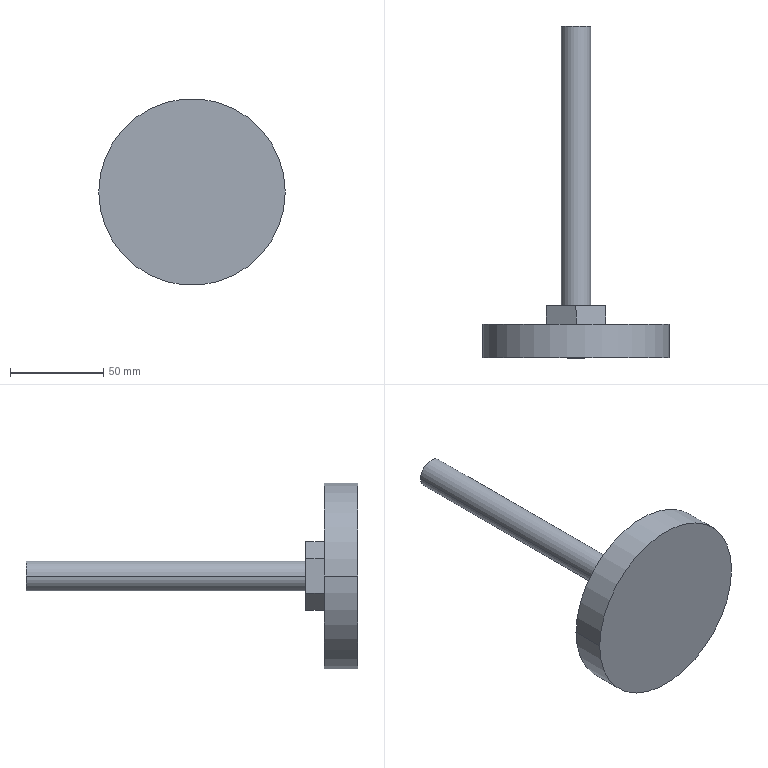Part | NX | 1 solid | 14 faces | box 100 x 178 x 100 mm | volume 180399 mm3 | plane 10 | cylinder 4 | commonest cylinder face diameters 16 x2 100 x2
STEP:
#1=CARTESIAN_POINT('',(-50.,-178.,0.));
#2=VERTEX_POINT('',#1);
#3=CARTESIAN_POINT('',(50.,-178.,0.));
#4=VERTEX_POINT('',#3);
#5=CARTESIAN_POINT('',(0.,-178.,0.));
#6=DIRECTION('',(0.,1.,0.));
#7=DIRECTION('',(1.,0.,0.));
#8=AXIS2_PLACEMENT_3D('',#5,#6,#7);
#9=CIRCLE('',#8,50.);
#10=EDGE_CURVE('',#2,#4,#9,.T.);
#11=ORIENTED_EDGE('',*,*,#10,.F.);
#12=CARTESIAN_POINT('',(0.,-178.,0.));
#13=DIRECTION('',(0.,1.,0.));
#14=DIRECTION('',(1.,0.,0.));
#15=AXIS2_PLACEMENT_3D('',#12,#13,#14);
#16=CIRCLE('',#15,50.);
#17=EDGE_CURVE('',#4,#2,#16,.T.);
#18=ORIENTED_EDGE('',*,*,#17,.F.);
#19=EDGE_LOOP('',(#11,#18));
#20=FACE_BOUND('',#19,.T.);
#21=CARTESIAN_POINT('',(0.,-178.,0.));
#22=DIRECTION('',(0.,1.,0.));
#23=DIRECTION('',(1.,0.,0.));
#24=AXIS2_PLACEMENT_3D('',#21,#22,#23);
#25=PLANE('',#24);
#26=ADVANCED_FACE('',(#20),#25,.F.);
#27=CARTESIAN_POINT('',(-50.,-160.,0.));
#28=VERTEX_POINT('',#27);
#29=CARTESIAN_POINT('',(50.,-160.,0.));
#30=VERTEX_POINT('',#29);
#31=CARTESIAN_POINT('',(0.,-160.,0.));
#32=DIRECTION('',(0.,1.,0.));
#33=DIRECTION('',(1.,0.,0.));
#34=AXIS2_PLACEMENT_3D('',#31,#32,#33);
#35=CIRCLE('',#34,50.);
#36=EDGE_CURVE('',#28,#30,#35,.T.);
#37=ORIENTED_EDGE('',*,*,#36,.F.);
#38=CARTESIAN_POINT('',(-50.,-189.,0.));
#39=DIRECTION('',(0.,1.,0.));
#40=VECTOR('',#39,1000.);
#41=LINE('',#38,#40);
#42=EDGE_CURVE('',#2,#28,#41,.T.);
#43=ORIENTED_EDGE('',*,*,#42,.F.);
#44=ORIENTED_EDGE('',*,*,#10,.T.);
#45=CARTESIAN_POINT('',(50.,-189.,0.));
#46=DIRECTION('',(0.,1.,0.));
#47=VECTOR('',#46,1000.);
#48=LINE('',#45,#47);
#49=EDGE_CURVE('',#4,#30,#48,.T.);
#50=ORIENTED_EDGE('',*,*,#49,.T.);
#51=EDGE_LOOP('',(#37,#43,#44,#50));
#52=FACE_BOUND('',#51,.T.);
#53=CARTESIAN_POINT('',(0.,-189.,0.));
#54=DIRECTION('',(0.,1.,0.));
#55=DIRECTION('',(1.,0.,0.));
#56=AXIS2_PLACEMENT_3D('',#53,#54,#55);
#57=CYLINDRICAL_SURFACE('',#56,50.);
#58=ADVANCED_FACE('',(#52),#57,.T.);
#59=CARTESIAN_POINT('',(8.,0.,0.));
#60=VERTEX_POINT('',#59);
#61=CARTESIAN_POINT('',(-8.,0.,0.));
#62=VERTEX_POINT('',#61);
#63=CARTESIAN_POINT('',(0.,0.,0.));
#64=DIRECTION('',(0.,-1.,0.));
#65=DIRECTION('',(-1.,0.,0.));
#66=AXIS2_PLACEMENT_3D('',#63,#64,#65);
#67=CIRCLE('',#66,8.);
#68=EDGE_CURVE('',#60,#62,#67,.T.);
#69=ORIENTED_EDGE('',*,*,#68,.F.);
#70=CARTESIAN_POINT('',(0.,0.,0.));
#71=DIRECTION('',(0.,-1.,0.));
#72=DIRECTION('',(-1.,0.,0.));
#73=AXIS2_PLACEMENT_3D('',#70,#71,#72);
#74=CIRCLE('',#73,8.);
#75=EDGE_CURVE('',#62,#60,#74,.T.);
#76=ORIENTED_EDGE('',*,*,#75,.F.);
#77=EDGE_LOOP('',(#69,#76));
#78=FACE_BOUND('',#77,.T.);
#79=CARTESIAN_POINT('',(0.,0.,0.));
#80=DIRECTION('',(0.,1.,0.));
#81=DIRECTION('',(1.,0.,0.));
#82=AXIS2_PLACEMENT_3D('',#79,#80,#81);
#83=PLANE('',#82);
#84=ADVANCED_FACE('',(#78),#83,.T.);
#85=ORIENTED_EDGE('',*,*,#36,.T.);
#86=CARTESIAN_POINT('',(0.,-160.,0.));
#87=DIRECTION('',(0.,1.,0.));
#88=DIRECTION('',(1.,0.,0.));
#89=AXIS2_PLACEMENT_3D('',#86,#87,#88);
#90=CIRCLE('',#89,50.);
#91=EDGE_CURVE('',#30,#28,#90,.T.);
#92=ORIENTED_EDGE('',*,*,#91,.T.);
#93=EDGE_LOOP('',(#85,#92));
#94=FACE_BOUND('',#93,.T.);
#95=CARTESIAN_POINT('',(0.,-160.,18.475));
#96=VERTEX_POINT('',#95);
#97=CARTESIAN_POINT('',(16.,-160.,9.238));
#98=VERTEX_POINT('',#97);
#99=CARTESIAN_POINT('',(0.,-160.,18.475));
#100=DIRECTION('',(0.866,0.,-0.5));
#101=VECTOR('',#100,1000.);
#102=LINE('',#99,#101);
#103=EDGE_CURVE('',#96,#98,#102,.T.);
#104=ORIENTED_EDGE('',*,*,#103,.F.);
#105=CARTESIAN_POINT('',(-16.,-160.,9.238));
#106=VERTEX_POINT('',#105);
#107=CARTESIAN_POINT('',(-16.,-160.,9.238));
#108=DIRECTION('',(0.866,0.,0.5));
#109=VECTOR('',#108,1000.);
#110=LINE('',#107,#109);
#111=EDGE_CURVE('',#106,#96,#110,.T.);
#112=ORIENTED_EDGE('',*,*,#111,.F.);
#113=CARTESIAN_POINT('',(-16.,-160.,-9.238));
#114=VERTEX_POINT('',#113);
#115=CARTESIAN_POINT('',(-16.,-160.,9.238));
#116=DIRECTION('',(0.,0.,-1.));
#117=VECTOR('',#116,1000.);
#118=LINE('',#115,#117);
#119=EDGE_CURVE('',#106,#114,#118,.T.);
#120=ORIENTED_EDGE('',*,*,#119,.T.);
#121=CARTESIAN_POINT('',(0.,-160.,-18.475));
#122=VERTEX_POINT('',#121);
#123=CARTESIAN_POINT('',(0.,-160.,-18.475));
#124=DIRECTION('',(-0.866,0.,0.5));
#125=VECTOR('',#124,1000.);
#126=LINE('',#123,#125);
#127=EDGE_CURVE('',#122,#114,#126,.T.);
#128=ORIENTED_EDGE('',*,*,#127,.F.);
#129=CARTESIAN_POINT('',(16.,-160.,-9.238));
#130=VERTEX_POINT('',#129);
#131=CARTESIAN_POINT('',(16.,-160.,-9.238));
#132=DIRECTION('',(-0.866,0.,-0.5));
#133=VECTOR('',#132,1000.);
#134=LINE('',#131,#133);
#135=EDGE_CURVE('',#130,#122,#134,.T.);
#136=ORIENTED_EDGE('',*,*,#135,.F.);
#137=CARTESIAN_POINT('',(16.,-160.,-9.238));
#138=DIRECTION('',(0.,0.,1.));
#139=VECTOR('',#138,1000.);
#140=LINE('',#137,#139);
#141=EDGE_CURVE('',#130,#98,#140,.T.);
#142=ORIENTED_EDGE('',*,*,#141,.T.);
#143=EDGE_LOOP('',(#104,#112,#120,#128,#136,#142));
#144=FACE_BOUND('',#143,.T.);
#145=CARTESIAN_POINT('',(0.,-160.,0.));
#146=DIRECTION('',(0.,1.,0.));
#147=DIRECTION('',(1.,0.,0.));
#148=AXIS2_PLACEMENT_3D('',#145,#146,#147);
#149=PLANE('',#148);
#150=ADVANCED_FACE('',(#94,#144),#149,.T.);
#151=ORIENTED_EDGE('',*,*,#103,.T.);
#152=CARTESIAN_POINT('',(16.,-150.,9.238));
#153=VERTEX_POINT('',#152);
#154=CARTESIAN_POINT('',(16.,-150.,9.238));
#155=DIRECTION('',(0.,-1.,0.));
#156=VECTOR('',#155,1000.);
#157=LINE('',#154,#156);
#158=EDGE_CURVE('',#153,#98,#157,.T.);
#159=ORIENTED_EDGE('',*,*,#158,.F.);
#160=CARTESIAN_POINT('',(0.,-150.,18.475));
#161=VERTEX_POINT('',#160);
#162=CARTESIAN_POINT('',(16.,-150.,9.238));
#163=DIRECTION('',(-0.866,0.,0.5));
#164=VECTOR('',#163,1000.);
#165=LINE('',#162,#164);
#166=EDGE_CURVE('',#153,#161,#165,.T.);
#167=ORIENTED_EDGE('',*,*,#166,.T.);
#168=CARTESIAN_POINT('',(0.,-150.,18.475));
#169=DIRECTION('',(0.,-1.,0.));
#170=VECTOR('',#169,1000.);
#171=LINE('',#168,#170);
#172=EDGE_CURVE('',#161,#96,#171,.T.);
#173=ORIENTED_EDGE('',*,*,#172,.T.);
#174=EDGE_LOOP('',(#151,#159,#167,#173));
#175=FACE_BOUND('',#174,.T.);
#176=CARTESIAN_POINT('',(0.,-160.,18.475));
#177=DIRECTION('',(0.5,0.,0.866));
#178=DIRECTION('',(0.,-1.,0.));
#179=AXIS2_PLACEMENT_3D('',#176,#177,#178);
#180=PLANE('',#179);
#181=ADVANCED_FACE('',(#175),#180,.T.);
#182=ORIENTED_EDGE('',*,*,#111,.T.);
#183=ORIENTED_EDGE('',*,*,#172,.F.);
#184=CARTESIAN_POINT('',(-16.,-150.,9.238));
#185=VERTEX_POINT('',#184);
#186=CARTESIAN_POINT('',(0.,-150.,18.475));
#187=DIRECTION('',(-0.866,0.,-0.5));
#188=VECTOR('',#187,1000.);
#189=LINE('',#186,#188);
#190=EDGE_CURVE('',#161,#185,#189,.T.);
#191=ORIENTED_EDGE('',*,*,#190,.T.);
#192=CARTESIAN_POINT('',(-16.,-150.,9.238));
#193=DIRECTION('',(0.,-1.,0.));
#194=VECTOR('',#193,1000.);
#195=LINE('',#192,#194);
#196=EDGE_CURVE('',#185,#106,#195,.T.);
#197=ORIENTED_EDGE('',*,*,#196,.T.);
#198=EDGE_LOOP('',(#182,#183,#191,#197));
#199=FACE_BOUND('',#198,.T.);
#200=CARTESIAN_POINT('',(-16.,-160.,9.238));
#201=DIRECTION('',(-0.5,0.,0.866));
#202=DIRECTION('',(0.,1.,0.));
#203=AXIS2_PLACEMENT_3D('',#200,#201,#202);
#204=PLANE('',#203);
#205=ADVANCED_FACE('',(#199),#204,.T.);
#206=ORIENTED_EDGE('',*,*,#119,.F.);
#207=ORIENTED_EDGE('',*,*,#196,.F.);
#208=CARTESIAN_POINT('',(-16.,-150.,-9.238));
#209=VERTEX_POINT('',#208);
#210=CARTESIAN_POINT('',(-16.,-150.,-9.238));
#211=DIRECTION('',(0.,0.,1.));
#212=VECTOR('',#211,1000.);
#213=LINE('',#210,#212);
#214=EDGE_CURVE('',#209,#185,#213,.T.);
#215=ORIENTED_EDGE('',*,*,#214,.F.);
#216=CARTESIAN_POINT('',(-16.,-150.,-9.238));
#217=DIRECTION('',(0.,-1.,0.));
#218=VECTOR('',#217,1000.);
#219=LINE('',#216,#218);
#220=EDGE_CURVE('',#209,#114,#219,.T.);
#221=ORIENTED_EDGE('',*,*,#220,.T.);
#222=EDGE_LOOP('',(#206,#207,#215,#221));
#223=FACE_BOUND('',#222,.T.);
#224=CARTESIAN_POINT('',(-16.,-160.,-9.238));
#225=DIRECTION('',(-1.,0.,0.));
#226=DIRECTION('',(0.,0.,1.));
#227=AXIS2_PLACEMENT_3D('',#224,#225,#226);
#228=PLANE('',#227);
#229=ADVANCED_FACE('',(#223),#228,.T.);
#230=ORIENTED_EDGE('',*,*,#127,.T.);
#231=ORIENTED_EDGE('',*,*,#220,.F.);
#232=CARTESIAN_POINT('',(0.,-150.,-18.475));
#233=VERTEX_POINT('',#232);
#234=CARTESIAN_POINT('',(-16.,-150.,-9.238));
#235=DIRECTION('',(0.866,0.,-0.5));
#236=VECTOR('',#235,1000.);
#237=LINE('',#234,#236);
#238=EDGE_CURVE('',#209,#233,#237,.T.);
#239=ORIENTED_EDGE('',*,*,#238,.T.);
#240=CARTESIAN_POINT('',(0.,-150.,-18.475));
#241=DIRECTION('',(0.,-1.,0.));
#242=VECTOR('',#241,1000.);
#243=LINE('',#240,#242);
#244=EDGE_CURVE('',#233,#122,#243,.T.);
#245=ORIENTED_EDGE('',*,*,#244,.T.);
#246=EDGE_LOOP('',(#230,#231,#239,#245));
#247=FACE_BOUND('',#246,.T.);
#248=CARTESIAN_POINT('',(0.,-160.,-18.475));
#249=DIRECTION('',(-0.5,0.,-0.866));
#250=DIRECTION('',(-0.866,0.,0.5));
#251=AXIS2_PLACEMENT_3D('',#248,#249,#250);
#252=PLANE('',#251);
#253=ADVANCED_FACE('',(#247),#252,.T.);
#254=ORIENTED_EDGE('',*,*,#135,.T.);
#255=ORIENTED_EDGE('',*,*,#244,.F.);
#256=CARTESIAN_POINT('',(16.,-150.,-9.238));
#257=VERTEX_POINT('',#256);
#258=CARTESIAN_POINT('',(0.,-150.,-18.475));
#259=DIRECTION('',(0.866,0.,0.5));
#260=VECTOR('',#259,1000.);
#261=LINE('',#258,#260);
#262=EDGE_CURVE('',#233,#257,#261,.T.);
#263=ORIENTED_EDGE('',*,*,#262,.T.);
#264=CARTESIAN_POINT('',(16.,-150.,-9.238));
#265=DIRECTION('',(0.,-1.,0.));
#266=VECTOR('',#265,1000.);
#267=LINE('',#264,#266);
#268=EDGE_CURVE('',#257,#130,#267,.T.);
#269=ORIENTED_EDGE('',*,*,#268,.T.);
#270=EDGE_LOOP('',(#254,#255,#263,#269));
#271=FACE_BOUND('',#270,.T.);
#272=CARTESIAN_POINT('',(16.,-160.,-9.238));
#273=DIRECTION('',(0.5,0.,-0.866));
#274=DIRECTION('',(0.,-1.,0.));
#275=AXIS2_PLACEMENT_3D('',#272,#273,#274);
#276=PLANE('',#275);
#277=ADVANCED_FACE('',(#271),#276,.T.);
#278=ORIENTED_EDGE('',*,*,#141,.F.);
#279=ORIENTED_EDGE('',*,*,#268,.F.);
#280=CARTESIAN_POINT('',(16.,-150.,9.238));
#281=DIRECTION('',(0.,0.,-1.));
#282=VECTOR('',#281,1000.);
#283=LINE('',#280,#282);
#284=EDGE_CURVE('',#153,#257,#283,.T.);
#285=ORIENTED_EDGE('',*,*,#284,.F.);
#286=ORIENTED_EDGE('',*,*,#158,.T.);
#287=EDGE_LOOP('',(#278,#279,#285,#286));
#288=FACE_BOUND('',#287,.T.);
#289=CARTESIAN_POINT('',(16.,-160.,9.238));
#290=DIRECTION('',(1.,0.,0.));
#291=DIRECTION('',(0.,1.,0.));
#292=AXIS2_PLACEMENT_3D('',#289,#290,#291);
#293=PLANE('',#292);
#294=ADVANCED_FACE('',(#288),#293,.T.);
#295=ORIENTED_EDGE('',*,*,#284,.T.);
#296=ORIENTED_EDGE('',*,*,#262,.F.);
#297=ORIENTED_EDGE('',*,*,#238,.F.);
#298=ORIENTED_EDGE('',*,*,#214,.T.);
#299=ORIENTED_EDGE('',*,*,#190,.F.);
#300=ORIENTED_EDGE('',*,*,#166,.F.);
#301=EDGE_LOOP('',(#295,#296,#297,#298,#299,#300));
#302=FACE_BOUND('',#301,.T.);
#303=CARTESIAN_POINT('',(-8.,-150.,0.));
#304=VERTEX_POINT('',#303);
#305=CARTESIAN_POINT('',(8.,-150.,0.));
#306=VERTEX_POINT('',#305);
#307=CARTESIAN_POINT('',(0.,-150.,0.));
#308=DIRECTION('',(0.,1.,0.));
#309=DIRECTION('',(-1.,0.,0.));
#310=AXIS2_PLACEMENT_3D('',#307,#308,#309);
#311=CIRCLE('',#310,8.);
#312=EDGE_CURVE('',#304,#306,#311,.T.);
#313=ORIENTED_EDGE('',*,*,#312,.F.);
#314=CARTESIAN_POINT('',(0.,-150.,0.));
#315=DIRECTION('',(0.,1.,0.));
#316=DIRECTION('',(-1.,0.,0.));
#317=AXIS2_PLACEMENT_3D('',#314,#315,#316);
#318=CIRCLE('',#317,8.);
#319=EDGE_CURVE('',#306,#304,#318,.T.);
#320=ORIENTED_EDGE('',*,*,#319,.F.);
#321=EDGE_LOOP('',(#313,#320));
#322=FACE_BOUND('',#321,.T.);
#323=CARTESIAN_POINT('',(0.,-150.,0.));
#324=DIRECTION('',(0.,1.,0.));
#325=DIRECTION('',(1.,0.,0.));
#326=AXIS2_PLACEMENT_3D('',#323,#324,#325);
#327=PLANE('',#326);
#328=ADVANCED_FACE('',(#302,#322),#327,.T.);
#329=ORIENTED_EDGE('',*,*,#68,.T.);
#330=CARTESIAN_POINT('',(-8.,-189.,0.));
#331=DIRECTION('',(0.,1.,0.));
#332=VECTOR('',#331,1000.);
#333=LINE('',#330,#332);
#334=EDGE_CURVE('',#304,#62,#333,.T.);
#335=ORIENTED_EDGE('',*,*,#334,.F.);
#336=ORIENTED_EDGE('',*,*,#312,.T.);
#337=CARTESIAN_POINT('',(8.,-189.,0.));
#338=DIRECTION('',(0.,1.,0.));
#339=VECTOR('',#338,1000.);
#340=LINE('',#337,#339);
#341=EDGE_CURVE('',#306,#60,#340,.T.);
#342=ORIENTED_EDGE('',*,*,#341,.T.);
#343=EDGE_LOOP('',(#329,#335,#336,#342));
#344=FACE_BOUND('',#343,.T.);
#345=CARTESIAN_POINT('',(0.,-189.,0.));
#346=DIRECTION('',(0.,1.,0.));
#347=DIRECTION('',(1.,0.,0.));
#348=AXIS2_PLACEMENT_3D('',#345,#346,#347);
#349=CYLINDRICAL_SURFACE('',#348,8.);
#350=ADVANCED_FACE('',(#344),#349,.T.);
#351=ORIENTED_EDGE('',*,*,#49,.F.);
#352=ORIENTED_EDGE('',*,*,#17,.T.);
#353=ORIENTED_EDGE('',*,*,#42,.T.);
#354=ORIENTED_EDGE('',*,*,#91,.F.);
#355=EDGE_LOOP('',(#351,#352,#353,#354));
#356=FACE_BOUND('',#355,.T.);
#357=CARTESIAN_POINT('',(0.,-189.,0.));
#358=DIRECTION('',(0.,1.,0.));
#359=DIRECTION('',(1.,0.,0.));
#360=AXIS2_PLACEMENT_3D('',#357,#358,#359);
#361=CYLINDRICAL_SURFACE('',#360,50.);
#362=ADVANCED_FACE('',(#356),#361,.T.);
#363=ORIENTED_EDGE('',*,*,#341,.F.);
#364=ORIENTED_EDGE('',*,*,#319,.T.);
#365=ORIENTED_EDGE('',*,*,#334,.T.);
#366=ORIENTED_EDGE('',*,*,#75,.T.);
#367=EDGE_LOOP('',(#363,#364,#365,#366));
#368=FACE_BOUND('',#367,.T.);
#369=CARTESIAN_POINT('',(0.,-189.,0.));
#370=DIRECTION('',(0.,1.,0.));
#371=DIRECTION('',(1.,0.,0.));
#372=AXIS2_PLACEMENT_3D('',#369,#370,#371);
#373=CYLINDRICAL_SURFACE('',#372,8.);
#374=ADVANCED_FACE('',(#368),#373,.T.);
#375=CLOSED_SHELL('',(#26,#58,#84,#150,#181,#205,#229,#253,#277,#294,#328,#350,#362,#374));
#376=MANIFOLD_SOLID_BREP('',#375);
#377=(LENGTH_UNIT()NAMED_UNIT(*)SI_UNIT(.MILLI.,.METRE.));
#378=UNCERTAINTY_MEASURE_WITH_UNIT(LENGTH_MEASURE(0.00001),#377,'','');
#379=(NAMED_UNIT(*)PLANE_ANGLE_UNIT()SI_UNIT($,.RADIAN.));
#380=(NAMED_UNIT(*)SI_UNIT($,.STERADIAN.)SOLID_ANGLE_UNIT());
#381=(GEOMETRIC_REPRESENTATION_CONTEXT(3)GLOBAL_UNCERTAINTY_ASSIGNED_CONTEXT((#378))GLOBAL_UNIT_ASSIGNED_CONTEXT((#377,#379,#380))REPRESENTATION_CONTEXT('',''));
#382=ADVANCED_BREP_SHAPE_REPRESENTATION('',(#376),#381);